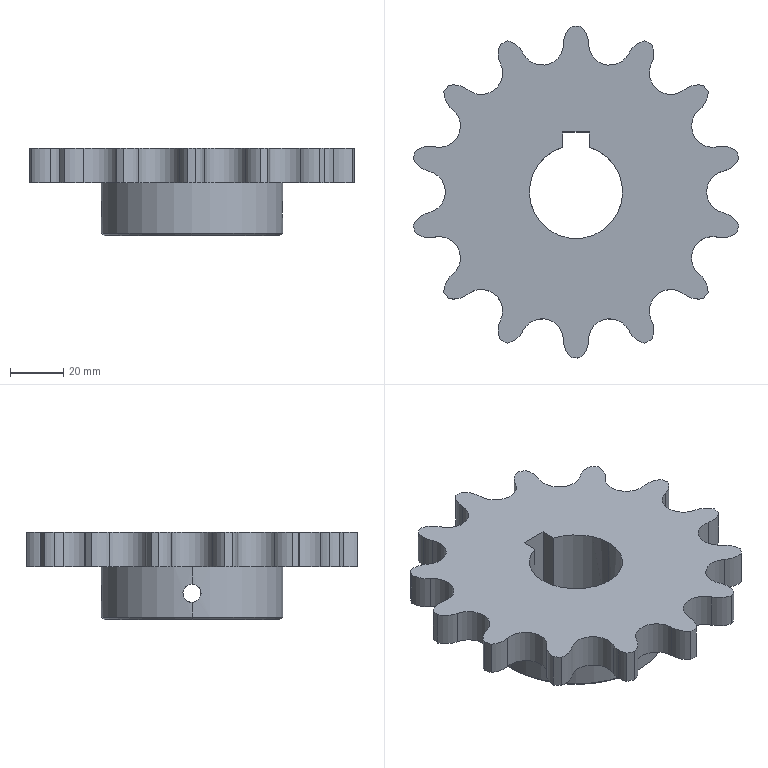Part | STEP file | 链轮-1 (2) | 1 solid | 84 faces | box 122.017 x 124.5 x 33 mm | volume 159053 mm3 | cylinder 76 | plane 6 | cone 2 | commonest cylinder face diameters 17.137 x31 16 x20 124.5 x14 6.8 x6 35 x3 68 x2